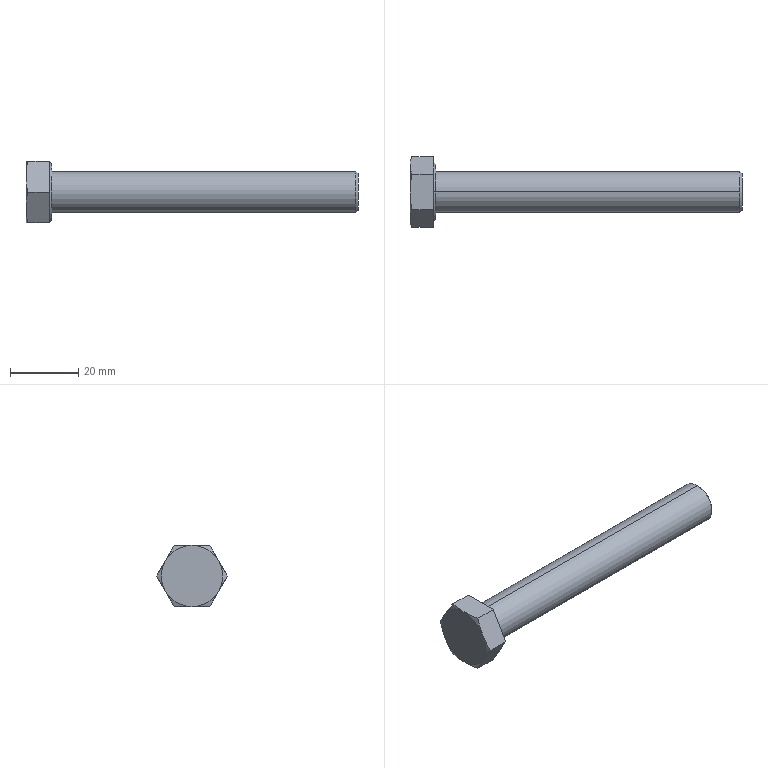Part | SolidWorks | features RevCut 3, Boss 1, Chamfer 1, Extrusion 1, Fillet 1, LPattern 1 | 1 solid | 22 faces | box 97.5 x 20.785 x 18 mm | volume 12242 mm3 | cone 10 | plane 10 | cylinder 2 | commonest cylinder face diameters 12 x2
STEP:
#1=CARTESIAN_POINT('',(97.5,0.,-5.4));
#2=VERTEX_POINT('',#1);
#3=CARTESIAN_POINT('',(97.5,0.,5.4));
#4=VERTEX_POINT('',#3);
#5=CARTESIAN_POINT('',(97.5,0.,0.));
#6=DIRECTION('',(1.,0.,0.));
#7=DIRECTION('',(0.,0.,-1.));
#8=AXIS2_PLACEMENT_3D('',#5,#6,#7);
#9=CIRCLE('',#8,5.4);
#10=EDGE_CURVE('',#2,#4,#9,.T.);
#11=ORIENTED_EDGE('',*,*,#10,.F.);
#12=CARTESIAN_POINT('',(96.9,0.,-6.));
#13=VERTEX_POINT('',#12);
#14=CARTESIAN_POINT('',(97.5,0.,-5.4));
#15=DIRECTION('',(-0.7071,0.,-0.7071));
#16=VECTOR('',#15,1000.);
#17=LINE('',#14,#16);
#18=EDGE_CURVE('',#2,#13,#17,.T.);
#19=ORIENTED_EDGE('',*,*,#18,.T.);
#20=CARTESIAN_POINT('',(96.9,0.,6.));
#21=VERTEX_POINT('',#20);
#22=CARTESIAN_POINT('',(96.9,0.,0.));
#23=DIRECTION('',(-1.,0.,0.));
#24=DIRECTION('',(0.,0.,-1.));
#25=AXIS2_PLACEMENT_3D('',#22,#23,#24);
#26=CIRCLE('',#25,6.);
#27=EDGE_CURVE('',#21,#13,#26,.T.);
#28=ORIENTED_EDGE('',*,*,#27,.F.);
#29=CARTESIAN_POINT('',(97.5,0.,5.4));
#30=DIRECTION('',(-0.7071,0.,0.7071));
#31=VECTOR('',#30,1000.);
#32=LINE('',#29,#31);
#33=EDGE_CURVE('',#4,#21,#32,.T.);
#34=ORIENTED_EDGE('',*,*,#33,.F.);
#35=EDGE_LOOP('',(#11,#19,#28,#34));
#36=FACE_OUTER_BOUND('',#35,.T.);
#37=CARTESIAN_POINT('',(97.5,0.,0.));
#38=DIRECTION('',(-1.,0.,0.));
#39=DIRECTION('',(0.,0.,1.));
#40=AXIS2_PLACEMENT_3D('',#37,#38,#39);
#41=CONICAL_SURFACE('',#40,5.4,0.7854);
#42=ADVANCED_FACE('',(#36),#41,.T.);
#43=ORIENTED_EDGE('',*,*,#27,.T.);
#44=CARTESIAN_POINT('',(7.5,0.,-6.));
#45=VERTEX_POINT('',#44);
#46=CARTESIAN_POINT('',(97.5,0.,-6.));
#47=DIRECTION('',(-1.,0.,0.));
#48=VECTOR('',#47,1000.);
#49=LINE('',#46,#48);
#50=EDGE_CURVE('',#13,#45,#49,.T.);
#51=ORIENTED_EDGE('',*,*,#50,.T.);
#52=CARTESIAN_POINT('',(7.5,0.,6.));
#53=VERTEX_POINT('',#52);
#54=CARTESIAN_POINT('',(7.5,0.,0.));
#55=DIRECTION('',(1.,0.,0.));
#56=DIRECTION('',(0.,0.,1.));
#57=AXIS2_PLACEMENT_3D('',#54,#55,#56);
#58=CIRCLE('',#57,6.);
#59=EDGE_CURVE('',#45,#53,#58,.T.);
#60=ORIENTED_EDGE('',*,*,#59,.T.);
#61=CARTESIAN_POINT('',(97.5,0.,6.));
#62=DIRECTION('',(-1.,0.,0.));
#63=VECTOR('',#62,1000.);
#64=LINE('',#61,#63);
#65=EDGE_CURVE('',#21,#53,#64,.T.);
#66=ORIENTED_EDGE('',*,*,#65,.F.);
#67=EDGE_LOOP('',(#43,#51,#60,#66));
#68=FACE_OUTER_BOUND('',#67,.T.);
#69=CARTESIAN_POINT('',(97.5,0.,0.));
#70=DIRECTION('',(-1.,0.,0.));
#71=DIRECTION('',(0.,0.,1.));
#72=AXIS2_PLACEMENT_3D('',#69,#70,#71);
#73=CYLINDRICAL_SURFACE('',#72,6.);
#74=ADVANCED_FACE('',(#68),#73,.T.);
#75=CARTESIAN_POINT('',(7.5,0.,8.235));
#76=VERTEX_POINT('',#75);
#77=CARTESIAN_POINT('',(7.5,0.,-8.235));
#78=VERTEX_POINT('',#77);
#79=CARTESIAN_POINT('',(7.5,0.,0.));
#80=DIRECTION('',(-1.,0.,0.));
#81=DIRECTION('',(0.,0.,1.));
#82=AXIS2_PLACEMENT_3D('',#79,#80,#81);
#83=CIRCLE('',#82,8.235);
#84=EDGE_CURVE('',#76,#78,#83,.T.);
#85=ORIENTED_EDGE('',*,*,#84,.T.);
#86=CARTESIAN_POINT('',(6.9,0.,-8.835));
#87=VERTEX_POINT('',#86);
#88=CARTESIAN_POINT('',(6.9,0.,-8.835));
#89=DIRECTION('',(-0.7071,0.,-0.7071));
#90=VECTOR('',#89,1000.);
#91=LINE('',#88,#90);
#92=EDGE_CURVE('',#78,#87,#91,.T.);
#93=ORIENTED_EDGE('',*,*,#92,.T.);
#94=CARTESIAN_POINT('',(6.9,0.,8.835));
#95=VERTEX_POINT('',#94);
#96=CARTESIAN_POINT('',(6.9,0.,0.));
#97=DIRECTION('',(-1.,0.,0.));
#98=DIRECTION('',(0.,0.,1.));
#99=AXIS2_PLACEMENT_3D('',#96,#97,#98);
#100=CIRCLE('',#99,8.835);
#101=EDGE_CURVE('',#95,#87,#100,.T.);
#102=ORIENTED_EDGE('',*,*,#101,.F.);
#103=CARTESIAN_POINT('',(6.9,0.,8.835));
#104=DIRECTION('',(-0.7071,0.,0.7071));
#105=VECTOR('',#104,1000.);
#106=LINE('',#103,#105);
#107=EDGE_CURVE('',#76,#95,#106,.T.);
#108=ORIENTED_EDGE('',*,*,#107,.F.);
#109=EDGE_LOOP('',(#85,#93,#102,#108));
#110=FACE_OUTER_BOUND('',#109,.T.);
#111=CARTESIAN_POINT('',(6.9,0.,0.));
#112=DIRECTION('',(-1.,0.,0.));
#113=DIRECTION('',(0.,0.,1.));
#114=AXIS2_PLACEMENT_3D('',#111,#112,#113);
#115=CONICAL_SURFACE('',#114,8.835,0.7854);
#116=ADVANCED_FACE('',(#110),#115,.T.);
#117=ORIENTED_EDGE('',*,*,#84,.F.);
#118=CARTESIAN_POINT('',(7.5,0.,0.));
#119=DIRECTION('',(-1.,0.,0.));
#120=DIRECTION('',(0.,0.,1.));
#121=AXIS2_PLACEMENT_3D('',#118,#119,#120);
#122=CIRCLE('',#121,8.235);
#123=EDGE_CURVE('',#78,#76,#122,.T.);
#124=ORIENTED_EDGE('',*,*,#123,.F.);
#125=EDGE_LOOP('',(#117,#124));
#126=FACE_OUTER_BOUND('',#125,.T.);
#127=CARTESIAN_POINT('',(7.5,0.,0.));
#128=DIRECTION('',(1.,0.,0.));
#129=DIRECTION('',(0.,0.,1.));
#130=AXIS2_PLACEMENT_3D('',#127,#128,#129);
#131=CIRCLE('',#130,6.);
#132=EDGE_CURVE('',#53,#45,#131,.T.);
#133=ORIENTED_EDGE('',*,*,#132,.F.);
#134=ORIENTED_EDGE('',*,*,#59,.F.);
#135=EDGE_LOOP('',(#133,#134));
#136=FACE_BOUND('',#135,.T.);
#137=CARTESIAN_POINT('',(7.5,-5.196,9.));
#138=DIRECTION('',(-1.,0.,0.));
#139=DIRECTION('',(0.,0.,1.));
#140=AXIS2_PLACEMENT_3D('',#137,#138,#139);
#141=PLANE('',#140);
#142=ADVANCED_FACE('',(#126,#136),#141,.F.);
#143=CARTESIAN_POINT('',(0.5068,-10.392,0.));
#144=VERTEX_POINT('',#143);
#145=CARTESIAN_POINT('',(0.,-7.794,4.5));
#146=VERTEX_POINT('',#145);
#147=CARTESIAN_POINT('',(0.5068,-10.392,0.));
#148=CARTESIAN_POINT('',(0.3492,-9.959,0.75));
#149=CARTESIAN_POINT('',(0.2212,-9.526,1.5));
#150=CARTESIAN_POINT('',(0.04634,-8.66,3.));
#151=CARTESIAN_POINT('',(0.,-8.227,3.75));
#152=CARTESIAN_POINT('',(0.,-7.794,4.5));
#153=B_SPLINE_CURVE_WITH_KNOTS('',3,(#147,#148,#149,#150,#151,#152),.UNSPECIFIED.,.F.,.F.,(4,2,4),(0.000000231,0.002598,0.005196),.UNSPECIFIED.);
#154=EDGE_CURVE('',#144,#146,#153,.T.);
#155=ORIENTED_EDGE('',*,*,#154,.F.);
#156=CARTESIAN_POINT('',(6.9,-10.392,0.));
#157=VERTEX_POINT('',#156);
#158=CARTESIAN_POINT('',(7.5,-10.392,0.));
#159=DIRECTION('',(-1.,0.,0.));
#160=VECTOR('',#159,1000.);
#161=LINE('',#158,#160);
#162=EDGE_CURVE('',#157,#144,#161,.T.);
#163=ORIENTED_EDGE('',*,*,#162,.F.);
#164=CARTESIAN_POINT('',(6.9,-5.196,9.));
#165=VERTEX_POINT('',#164);
#166=CARTESIAN_POINT('',(6.9,-5.196,9.));
#167=DIRECTION('',(0.,-0.5,-0.866));
#168=VECTOR('',#167,1000.);
#169=LINE('',#166,#168);
#170=EDGE_CURVE('',#165,#157,#169,.T.);
#171=ORIENTED_EDGE('',*,*,#170,.F.);
#172=CARTESIAN_POINT('',(0.5068,-5.196,9.));
#173=VERTEX_POINT('',#172);
#174=CARTESIAN_POINT('',(7.5,-5.196,9.));
#175=DIRECTION('',(-1.,0.,0.));
#176=VECTOR('',#175,1000.);
#177=LINE('',#174,#176);
#178=EDGE_CURVE('',#165,#173,#177,.T.);
#179=ORIENTED_EDGE('',*,*,#178,.T.);
#180=CARTESIAN_POINT('',(0.,-7.794,4.5));
#181=CARTESIAN_POINT('',(0.,-7.361,5.25));
#182=CARTESIAN_POINT('',(0.04634,-6.928,6.));
#183=CARTESIAN_POINT('',(0.2212,-6.062,7.5));
#184=CARTESIAN_POINT('',(0.3492,-5.629,8.25));
#185=CARTESIAN_POINT('',(0.5068,-5.196,9.));
#186=B_SPLINE_CURVE_WITH_KNOTS('',3,(#180,#181,#182,#183,#184,#185),.UNSPECIFIED.,.F.,.F.,(4,2,4),(0.005196,0.007794,0.01039),.UNSPECIFIED.);
#187=EDGE_CURVE('',#146,#173,#186,.T.);
#188=ORIENTED_EDGE('',*,*,#187,.F.);
#189=EDGE_LOOP('',(#155,#163,#171,#179,#188));
#190=FACE_OUTER_BOUND('',#189,.T.);
#191=CARTESIAN_POINT('',(7.5,-5.196,9.));
#192=DIRECTION('',(0.,0.866,-0.5));
#193=DIRECTION('',(0.,0.5,0.866));
#194=AXIS2_PLACEMENT_3D('',#191,#192,#193);
#195=PLANE('',#194);
#196=ADVANCED_FACE('',(#190),#195,.F.);
#197=CARTESIAN_POINT('',(0.5068,-5.196,-9.));
#198=VERTEX_POINT('',#197);
#199=CARTESIAN_POINT('',(0.,-7.794,-4.5));
#200=VERTEX_POINT('',#199);
#201=CARTESIAN_POINT('',(0.5068,-5.196,-9.));
#202=CARTESIAN_POINT('',(0.3492,-5.629,-8.25));
#203=CARTESIAN_POINT('',(0.2212,-6.062,-7.5));
#204=CARTESIAN_POINT('',(0.04634,-6.928,-6.));
#205=CARTESIAN_POINT('',(0.,-7.361,-5.25));
#206=CARTESIAN_POINT('',(0.,-7.794,-4.5));
#207=B_SPLINE_CURVE_WITH_KNOTS('',3,(#201,#202,#203,#204,#205,#206),.UNSPECIFIED.,.F.,.F.,(4,2,4),(0.000000231,0.002598,0.005196),.UNSPECIFIED.);
#208=EDGE_CURVE('',#198,#200,#207,.T.);
#209=ORIENTED_EDGE('',*,*,#208,.F.);
#210=CARTESIAN_POINT('',(6.9,-5.196,-9.));
#211=VERTEX_POINT('',#210);
#212=CARTESIAN_POINT('',(7.5,-5.196,-9.));
#213=DIRECTION('',(-1.,0.,0.));
#214=VECTOR('',#213,1000.);
#215=LINE('',#212,#214);
#216=EDGE_CURVE('',#211,#198,#215,.T.);
#217=ORIENTED_EDGE('',*,*,#216,.F.);
#218=CARTESIAN_POINT('',(6.9,-10.392,0.));
#219=DIRECTION('',(0.,0.5,-0.866));
#220=VECTOR('',#219,1000.);
#221=LINE('',#218,#220);
#222=EDGE_CURVE('',#157,#211,#221,.T.);
#223=ORIENTED_EDGE('',*,*,#222,.F.);
#224=ORIENTED_EDGE('',*,*,#162,.T.);
#225=CARTESIAN_POINT('',(0.,-7.794,-4.5));
#226=CARTESIAN_POINT('',(0.,-8.227,-3.75));
#227=CARTESIAN_POINT('',(0.04634,-8.66,-3.));
#228=CARTESIAN_POINT('',(0.2212,-9.526,-1.5));
#229=CARTESIAN_POINT('',(0.3492,-9.959,-0.75));
#230=CARTESIAN_POINT('',(0.5068,-10.392,0.));
#231=B_SPLINE_CURVE_WITH_KNOTS('',3,(#225,#226,#227,#228,#229,#230),.UNSPECIFIED.,.F.,.F.,(4,2,4),(0.005196,0.007794,0.01039),.UNSPECIFIED.);
#232=EDGE_CURVE('',#200,#144,#231,.T.);
#233=ORIENTED_EDGE('',*,*,#232,.F.);
#234=EDGE_LOOP('',(#209,#217,#223,#224,#233));
#235=FACE_OUTER_BOUND('',#234,.T.);
#236=CARTESIAN_POINT('',(7.5,-10.392,0.));
#237=DIRECTION('',(0.,0.866,0.5));
#238=DIRECTION('',(0.,-0.5,0.866));
#239=AXIS2_PLACEMENT_3D('',#236,#237,#238);
#240=PLANE('',#239);
#241=ADVANCED_FACE('',(#235),#240,.F.);
#242=CARTESIAN_POINT('',(0.5068,5.196,-9.));
#243=VERTEX_POINT('',#242);
#244=CARTESIAN_POINT('',(0.,0.,-9.));
#245=VERTEX_POINT('',#244);
#246=CARTESIAN_POINT('',(0.5068,5.196,-9.));
#247=CARTESIAN_POINT('',(0.3496,4.332,-9.));
#248=CARTESIAN_POINT('',(0.2215,3.467,-9.));
#249=CARTESIAN_POINT('',(0.04652,1.735,-9.));
#250=CARTESIAN_POINT('',(0.,0.8678,-9.));
#251=CARTESIAN_POINT('',(0.,0.,-9.));
#252=B_SPLINE_CURVE_WITH_KNOTS('',3,(#246,#247,#248,#249,#250,#251),.UNSPECIFIED.,.F.,.F.,(4,2,4),(0.01874,0.02136,0.02398),.UNSPECIFIED.);
#253=EDGE_CURVE('',#243,#245,#252,.T.);
#254=ORIENTED_EDGE('',*,*,#253,.F.);
#255=CARTESIAN_POINT('',(6.9,5.196,-9.));
#256=VERTEX_POINT('',#255);
#257=CARTESIAN_POINT('',(7.5,5.196,-9.));
#258=DIRECTION('',(-1.,0.,0.));
#259=VECTOR('',#258,1000.);
#260=LINE('',#257,#259);
#261=EDGE_CURVE('',#256,#243,#260,.T.);
#262=ORIENTED_EDGE('',*,*,#261,.F.);
#263=CARTESIAN_POINT('',(6.9,-5.196,-9.));
#264=DIRECTION('',(0.,1.,0.));
#265=VECTOR('',#264,1000.);
#266=LINE('',#263,#265);
#267=EDGE_CURVE('',#211,#256,#266,.T.);
#268=ORIENTED_EDGE('',*,*,#267,.F.);
#269=ORIENTED_EDGE('',*,*,#216,.T.);
#270=CARTESIAN_POINT('',(0.,0.,-9.));
#271=CARTESIAN_POINT('',(0.,-0.8653,-9.));
#272=CARTESIAN_POINT('',(0.04627,-1.732,-9.));
#273=CARTESIAN_POINT('',(0.2214,-3.466,-9.));
#274=CARTESIAN_POINT('',(0.3502,-4.336,-9.));
#275=CARTESIAN_POINT('',(0.5068,-5.196,-9.));
#276=B_SPLINE_CURVE_WITH_KNOTS('',3,(#270,#271,#272,#273,#274,#275),.UNSPECIFIED.,.F.,.F.,(4,2,4),(0.02398,0.02659,0.0292),.UNSPECIFIED.);
#277=EDGE_CURVE('',#245,#198,#276,.T.);
#278=ORIENTED_EDGE('',*,*,#277,.F.);
#279=EDGE_LOOP('',(#254,#262,#268,#269,#278));
#280=FACE_OUTER_BOUND('',#279,.T.);
#281=CARTESIAN_POINT('',(7.5,-5.196,-9.));
#282=DIRECTION('',(0.,0.,1.));
#283=DIRECTION('',(0.,-1.,0.));
#284=AXIS2_PLACEMENT_3D('',#281,#282,#283);
#285=PLANE('',#284);
#286=ADVANCED_FACE('',(#280),#285,.F.);
#287=CARTESIAN_POINT('',(0.5068,10.392,0.));
#288=VERTEX_POINT('',#287);
#289=CARTESIAN_POINT('',(0.,7.794,-4.5));
#290=VERTEX_POINT('',#289);
#291=CARTESIAN_POINT('',(0.5068,10.392,0.));
#292=CARTESIAN_POINT('',(0.3492,9.959,-0.75));
#293=CARTESIAN_POINT('',(0.2212,9.526,-1.5));
#294=CARTESIAN_POINT('',(0.04634,8.66,-3.));
#295=CARTESIAN_POINT('',(0.,8.227,-3.75));
#296=CARTESIAN_POINT('',(0.,7.794,-4.5));
#297=B_SPLINE_CURVE_WITH_KNOTS('',3,(#291,#292,#293,#294,#295,#296),.UNSPECIFIED.,.F.,.F.,(4,2,4),(0.000000231,0.002598,0.005196),.UNSPECIFIED.);
#298=EDGE_CURVE('',#288,#290,#297,.T.);
#299=ORIENTED_EDGE('',*,*,#298,.F.);
#300=CARTESIAN_POINT('',(6.9,10.392,0.));
#301=VERTEX_POINT('',#300);
#302=CARTESIAN_POINT('',(7.5,10.392,0.));
#303=DIRECTION('',(-1.,0.,0.));
#304=VECTOR('',#303,1000.);
#305=LINE('',#302,#304);
#306=EDGE_CURVE('',#301,#288,#305,.T.);
#307=ORIENTED_EDGE('',*,*,#306,.F.);
#308=CARTESIAN_POINT('',(6.9,5.196,-9.));
#309=DIRECTION('',(0.,0.5,0.866));
#310=VECTOR('',#309,1000.);
#311=LINE('',#308,#310);
#312=EDGE_CURVE('',#256,#301,#311,.T.);
#313=ORIENTED_EDGE('',*,*,#312,.F.);
#314=ORIENTED_EDGE('',*,*,#261,.T.);
#315=CARTESIAN_POINT('',(0.,7.794,-4.5));
#316=CARTESIAN_POINT('',(0.,7.361,-5.25));
#317=CARTESIAN_POINT('',(0.04634,6.928,-6.));
#318=CARTESIAN_POINT('',(0.2212,6.062,-7.5));
#319=CARTESIAN_POINT('',(0.3492,5.629,-8.25));
#320=CARTESIAN_POINT('',(0.5068,5.196,-9.));
#321=B_SPLINE_CURVE_WITH_KNOTS('',3,(#315,#316,#317,#318,#319,#320),.UNSPECIFIED.,.F.,.F.,(4,2,4),(0.005196,0.007794,0.01039),.UNSPECIFIED.);
#322=EDGE_CURVE('',#290,#243,#321,.T.);
#323=ORIENTED_EDGE('',*,*,#322,.F.);
#324=EDGE_LOOP('',(#299,#307,#313,#314,#323));
#325=FACE_OUTER_BOUND('',#324,.T.);
#326=CARTESIAN_POINT('',(7.5,5.196,-9.));
#327=DIRECTION('',(0.,-0.866,0.5));
#328=DIRECTION('',(0.,-0.5,-0.866));
#329=AXIS2_PLACEMENT_3D('',#326,#327,#328);
#330=PLANE('',#329);
#331=ADVANCED_FACE('',(#325),#330,.F.);
#332=CARTESIAN_POINT('',(0.5068,5.196,9.));
#333=VERTEX_POINT('',#332);
#334=CARTESIAN_POINT('',(0.,7.794,4.5));
#335=VERTEX_POINT('',#334);
#336=CARTESIAN_POINT('',(0.5068,5.196,9.));
#337=CARTESIAN_POINT('',(0.3492,5.629,8.25));
#338=CARTESIAN_POINT('',(0.2212,6.062,7.5));
#339=CARTESIAN_POINT('',(0.04634,6.928,6.));
#340=CARTESIAN_POINT('',(0.,7.361,5.25));
#341=CARTESIAN_POINT('',(0.,7.794,4.5));
#342=B_SPLINE_CURVE_WITH_KNOTS('',3,(#336,#337,#338,#339,#340,#341),.UNSPECIFIED.,.F.,.F.,(4,2,4),(0.000000231,0.002598,0.005196),.UNSPECIFIED.);
#343=EDGE_CURVE('',#333,#335,#342,.T.);
#344=ORIENTED_EDGE('',*,*,#343,.F.);
#345=CARTESIAN_POINT('',(6.9,5.196,9.));
#346=VERTEX_POINT('',#345);
#347=CARTESIAN_POINT('',(7.5,5.196,9.));
#348=DIRECTION('',(-1.,0.,0.));
#349=VECTOR('',#348,1000.);
#350=LINE('',#347,#349);
#351=EDGE_CURVE('',#346,#333,#350,.T.);
#352=ORIENTED_EDGE('',*,*,#351,.F.);
#353=CARTESIAN_POINT('',(6.9,10.392,0.));
#354=DIRECTION('',(0.,-0.5,0.866));
#355=VECTOR('',#354,1000.);
#356=LINE('',#353,#355);
#357=EDGE_CURVE('',#301,#346,#356,.T.);
#358=ORIENTED_EDGE('',*,*,#357,.F.);
#359=ORIENTED_EDGE('',*,*,#306,.T.);
#360=CARTESIAN_POINT('',(0.,7.794,4.5));
#361=CARTESIAN_POINT('',(0.,8.227,3.75));
#362=CARTESIAN_POINT('',(0.04634,8.66,3.));
#363=CARTESIAN_POINT('',(0.2212,9.526,1.5));
#364=CARTESIAN_POINT('',(0.3492,9.959,0.75));
#365=CARTESIAN_POINT('',(0.5068,10.392,0.));
#366=B_SPLINE_CURVE_WITH_KNOTS('',3,(#360,#361,#362,#363,#364,#365),.UNSPECIFIED.,.F.,.F.,(4,2,4),(0.005196,0.007794,0.01039),.UNSPECIFIED.);
#367=EDGE_CURVE('',#335,#288,#366,.T.);
#368=ORIENTED_EDGE('',*,*,#367,.F.);
#369=EDGE_LOOP('',(#344,#352,#358,#359,#368));
#370=FACE_OUTER_BOUND('',#369,.T.);
#371=CARTESIAN_POINT('',(7.5,10.392,0.));
#372=DIRECTION('',(0.,-0.866,-0.5));
#373=DIRECTION('',(0.,0.5,-0.866));
#374=AXIS2_PLACEMENT_3D('',#371,#372,#373);
#375=PLANE('',#374);
#376=ADVANCED_FACE('',(#370),#375,.F.);
#377=CARTESIAN_POINT('',(0.,0.,9.));
#378=VERTEX_POINT('',#377);
#379=CARTESIAN_POINT('',(0.5068,-5.196,9.));
#380=CARTESIAN_POINT('',(0.3502,-4.336,9.));
#381=CARTESIAN_POINT('',(0.2214,-3.466,9.));
#382=CARTESIAN_POINT('',(0.04627,-1.732,9.));
#383=CARTESIAN_POINT('',(0.,-0.8653,9.));
#384=CARTESIAN_POINT('',(0.,0.,9.));
#385=B_SPLINE_CURVE_WITH_KNOTS('',3,(#379,#380,#381,#382,#383,#384),.UNSPECIFIED.,.F.,.F.,(4,2,4),(0.008839,0.01146,0.01408),.UNSPECIFIED.);
#386=EDGE_CURVE('',#173,#378,#385,.T.);
#387=ORIENTED_EDGE('',*,*,#386,.F.);
#388=ORIENTED_EDGE('',*,*,#178,.F.);
#389=CARTESIAN_POINT('',(6.9,5.196,9.));
#390=DIRECTION('',(0.,-1.,0.));
#391=VECTOR('',#390,1000.);
#392=LINE('',#389,#391);
#393=EDGE_CURVE('',#346,#165,#392,.T.);
#394=ORIENTED_EDGE('',*,*,#393,.F.);
#395=ORIENTED_EDGE('',*,*,#351,.T.);
#396=CARTESIAN_POINT('',(0.,0.,9.));
#397=CARTESIAN_POINT('',(0.,0.8678,9.));
#398=CARTESIAN_POINT('',(0.04652,1.735,9.));
#399=CARTESIAN_POINT('',(0.2215,3.467,9.));
#400=CARTESIAN_POINT('',(0.3496,4.332,9.));
#401=CARTESIAN_POINT('',(0.5068,5.196,9.));
#402=B_SPLINE_CURVE_WITH_KNOTS('',3,(#396,#397,#398,#399,#400,#401),.UNSPECIFIED.,.F.,.F.,(4,2,4),(0.01408,0.0167,0.01933),.UNSPECIFIED.);
#403=EDGE_CURVE('',#378,#333,#402,.T.);
#404=ORIENTED_EDGE('',*,*,#403,.F.);
#405=EDGE_LOOP('',(#387,#388,#394,#395,#404));
#406=FACE_OUTER_BOUND('',#405,.T.);
#407=CARTESIAN_POINT('',(7.5,5.196,9.));
#408=DIRECTION('',(0.,0.,-1.));
#409=DIRECTION('',(-1.,0.,0.));
#410=AXIS2_PLACEMENT_3D('',#407,#408,#409);
#411=PLANE('',#410);
#412=ADVANCED_FACE('',(#406),#411,.F.);
#413=ORIENTED_EDGE('',*,*,#101,.T.);
#414=CARTESIAN_POINT('',(6.9,0.,0.));
#415=DIRECTION('',(-1.,0.,0.));
#416=DIRECTION('',(0.,0.,1.));
#417=AXIS2_PLACEMENT_3D('',#414,#415,#416);
#418=CIRCLE('',#417,8.835);
#419=EDGE_CURVE('',#87,#95,#418,.T.);
#420=ORIENTED_EDGE('',*,*,#419,.T.);
#421=EDGE_LOOP('',(#413,#420));
#422=FACE_BOUND('',#421,.T.);
#423=ORIENTED_EDGE('',*,*,#170,.T.);
#424=ORIENTED_EDGE('',*,*,#222,.T.);
#425=ORIENTED_EDGE('',*,*,#267,.T.);
#426=ORIENTED_EDGE('',*,*,#312,.T.);
#427=ORIENTED_EDGE('',*,*,#357,.T.);
#428=ORIENTED_EDGE('',*,*,#393,.T.);
#429=EDGE_LOOP('',(#423,#424,#425,#426,#427,#428));
#430=FACE_OUTER_BOUND('',#429,.T.);
#431=CARTESIAN_POINT('',(6.9,8.835,0.));
#432=DIRECTION('',(1.,0.,0.));
#433=DIRECTION('',(0.,0.,-1.));
#434=AXIS2_PLACEMENT_3D('',#431,#432,#433);
#435=PLANE('',#434);
#436=ADVANCED_FACE('',(#422,#430),#435,.T.);
#437=ORIENTED_EDGE('',*,*,#92,.F.);
#438=ORIENTED_EDGE('',*,*,#123,.T.);
#439=ORIENTED_EDGE('',*,*,#107,.T.);
#440=ORIENTED_EDGE('',*,*,#419,.F.);
#441=EDGE_LOOP('',(#437,#438,#439,#440));
#442=FACE_OUTER_BOUND('',#441,.T.);
#443=CARTESIAN_POINT('',(6.9,0.,0.));
#444=DIRECTION('',(-1.,0.,0.));
#445=DIRECTION('',(0.,0.,1.));
#446=AXIS2_PLACEMENT_3D('',#443,#444,#445);
#447=CONICAL_SURFACE('',#446,8.835,0.7854);
#448=ADVANCED_FACE('',(#442),#447,.T.);
#449=ORIENTED_EDGE('',*,*,#187,.T.);
#450=ORIENTED_EDGE('',*,*,#386,.T.);
#451=CARTESIAN_POINT('',(0.,0.,0.));
#452=DIRECTION('',(-1.,0.,0.));
#453=DIRECTION('',(0.,0.,1.));
#454=AXIS2_PLACEMENT_3D('',#451,#452,#453);
#455=CIRCLE('',#454,9.);
#456=EDGE_CURVE('',#146,#378,#455,.T.);
#457=ORIENTED_EDGE('',*,*,#456,.F.);
#458=EDGE_LOOP('',(#449,#450,#457));
#459=FACE_OUTER_BOUND('',#458,.T.);
#460=CARTESIAN_POINT('',(0.,0.,0.));
#461=DIRECTION('',(1.,0.,0.));
#462=DIRECTION('',(0.,0.,-1.));
#463=AXIS2_PLACEMENT_3D('',#460,#461,#462);
#464=CONICAL_SURFACE('',#463,9.,1.222);
#465=ADVANCED_FACE('',(#459),#464,.T.);
#466=ORIENTED_EDGE('',*,*,#232,.T.);
#467=ORIENTED_EDGE('',*,*,#154,.T.);
#468=CARTESIAN_POINT('',(0.,0.,0.));
#469=DIRECTION('',(-1.,0.,0.));
#470=DIRECTION('',(0.,0.,1.));
#471=AXIS2_PLACEMENT_3D('',#468,#469,#470);
#472=CIRCLE('',#471,9.);
#473=EDGE_CURVE('',#200,#146,#472,.T.);
#474=ORIENTED_EDGE('',*,*,#473,.F.);
#475=EDGE_LOOP('',(#466,#467,#474));
#476=FACE_OUTER_BOUND('',#475,.T.);
#477=CARTESIAN_POINT('',(0.,0.,0.));
#478=DIRECTION('',(1.,0.,0.));
#479=DIRECTION('',(0.,0.,-1.));
#480=AXIS2_PLACEMENT_3D('',#477,#478,#479);
#481=CONICAL_SURFACE('',#480,9.,1.222);
#482=ADVANCED_FACE('',(#476),#481,.T.);
#483=ORIENTED_EDGE('',*,*,#277,.T.);
#484=ORIENTED_EDGE('',*,*,#208,.T.);
#485=CARTESIAN_POINT('',(0.,0.,0.));
#486=DIRECTION('',(-1.,0.,0.));
#487=DIRECTION('',(0.,0.,1.));
#488=AXIS2_PLACEMENT_3D('',#485,#486,#487);
#489=CIRCLE('',#488,9.);
#490=EDGE_CURVE('',#245,#200,#489,.T.);
#491=ORIENTED_EDGE('',*,*,#490,.F.);
#492=EDGE_LOOP('',(#483,#484,#491));
#493=FACE_OUTER_BOUND('',#492,.T.);
#494=CARTESIAN_POINT('',(0.,0.,0.));
#495=DIRECTION('',(1.,0.,0.));
#496=DIRECTION('',(0.,0.,-1.));
#497=AXIS2_PLACEMENT_3D('',#494,#495,#496);
#498=CONICAL_SURFACE('',#497,9.,1.222);
#499=ADVANCED_FACE('',(#493),#498,.T.);
#500=ORIENTED_EDGE('',*,*,#253,.T.);
#501=CARTESIAN_POINT('',(0.,0.,0.));
#502=DIRECTION('',(-1.,0.,0.));
#503=DIRECTION('',(0.,0.,1.));
#504=AXIS2_PLACEMENT_3D('',#501,#502,#503);
#505=CIRCLE('',#504,9.);
#506=EDGE_CURVE('',#290,#245,#505,.T.);
#507=ORIENTED_EDGE('',*,*,#506,.F.);
#508=ORIENTED_EDGE('',*,*,#322,.T.);
#509=EDGE_LOOP('',(#500,#507,#508));
#510=FACE_OUTER_BOUND('',#509,.T.);
#511=CARTESIAN_POINT('',(0.,0.,0.));
#512=DIRECTION('',(1.,0.,0.));
#513=DIRECTION('',(0.,0.,-1.));
#514=AXIS2_PLACEMENT_3D('',#511,#512,#513);
#515=CONICAL_SURFACE('',#514,9.,1.222);
#516=ADVANCED_FACE('',(#510),#515,.T.);
#517=ORIENTED_EDGE('',*,*,#298,.T.);
#518=CARTESIAN_POINT('',(0.,0.,0.));
#519=DIRECTION('',(-1.,0.,0.));
#520=DIRECTION('',(0.,0.,1.));
#521=AXIS2_PLACEMENT_3D('',#518,#519,#520);
#522=CIRCLE('',#521,9.);
#523=EDGE_CURVE('',#335,#290,#522,.T.);
#524=ORIENTED_EDGE('',*,*,#523,.F.);
#525=ORIENTED_EDGE('',*,*,#367,.T.);
#526=EDGE_LOOP('',(#517,#524,#525));
#527=FACE_OUTER_BOUND('',#526,.T.);
#528=CARTESIAN_POINT('',(0.,0.,0.));
#529=DIRECTION('',(1.,0.,0.));
#530=DIRECTION('',(0.,0.,-1.));
#531=AXIS2_PLACEMENT_3D('',#528,#529,#530);
#532=CONICAL_SURFACE('',#531,9.,1.222);
#533=ADVANCED_FACE('',(#527),#532,.T.);
#534=ORIENTED_EDGE('',*,*,#343,.T.);
#535=CARTESIAN_POINT('',(0.,0.,0.));
#536=DIRECTION('',(-1.,0.,0.));
#537=DIRECTION('',(0.,0.,1.));
#538=AXIS2_PLACEMENT_3D('',#535,#536,#537);
#539=CIRCLE('',#538,9.);
#540=EDGE_CURVE('',#378,#335,#539,.T.);
#541=ORIENTED_EDGE('',*,*,#540,.F.);
#542=ORIENTED_EDGE('',*,*,#403,.T.);
#543=EDGE_LOOP('',(#534,#541,#542));
#544=FACE_OUTER_BOUND('',#543,.T.);
#545=CARTESIAN_POINT('',(0.,0.,0.));
#546=DIRECTION('',(1.,0.,0.));
#547=DIRECTION('',(0.,0.,-1.));
#548=AXIS2_PLACEMENT_3D('',#545,#546,#547);
#549=CONICAL_SURFACE('',#548,9.,1.222);
#550=ADVANCED_FACE('',(#544),#549,.T.);
#551=ORIENTED_EDGE('',*,*,#456,.T.);
#552=ORIENTED_EDGE('',*,*,#540,.T.);
#553=ORIENTED_EDGE('',*,*,#523,.T.);
#554=ORIENTED_EDGE('',*,*,#506,.T.);
#555=ORIENTED_EDGE('',*,*,#490,.T.);
#556=ORIENTED_EDGE('',*,*,#473,.T.);
#557=EDGE_LOOP('',(#551,#552,#553,#554,#555,#556));
#558=FACE_OUTER_BOUND('',#557,.T.);
#559=CARTESIAN_POINT('',(0.,-5.196,9.));
#560=DIRECTION('',(-1.,0.,0.));
#561=DIRECTION('',(0.,0.,1.));
#562=AXIS2_PLACEMENT_3D('',#559,#560,#561);
#563=PLANE('',#562);
#564=ADVANCED_FACE('',(#558),#563,.T.);
#565=ORIENTED_EDGE('',*,*,#50,.F.);
#566=CARTESIAN_POINT('',(96.9,0.,0.));
#567=DIRECTION('',(-1.,0.,0.));
#568=DIRECTION('',(0.,0.,-1.));
#569=AXIS2_PLACEMENT_3D('',#566,#567,#568);
#570=CIRCLE('',#569,6.);
#571=EDGE_CURVE('',#13,#21,#570,.T.);
#572=ORIENTED_EDGE('',*,*,#571,.T.);
#573=ORIENTED_EDGE('',*,*,#65,.T.);
#574=ORIENTED_EDGE('',*,*,#132,.T.);
#575=EDGE_LOOP('',(#565,#572,#573,#574));
#576=FACE_OUTER_BOUND('',#575,.T.);
#577=CARTESIAN_POINT('',(97.5,0.,0.));
#578=DIRECTION('',(-1.,0.,0.));
#579=DIRECTION('',(0.,0.,1.));
#580=AXIS2_PLACEMENT_3D('',#577,#578,#579);
#581=CYLINDRICAL_SURFACE('',#580,6.);
#582=ADVANCED_FACE('',(#576),#581,.T.);
#583=CARTESIAN_POINT('',(97.5,0.,0.));
#584=DIRECTION('',(1.,0.,0.));
#585=DIRECTION('',(0.,0.,-1.));
#586=AXIS2_PLACEMENT_3D('',#583,#584,#585);
#587=CIRCLE('',#586,5.4);
#588=EDGE_CURVE('',#4,#2,#587,.T.);
#589=ORIENTED_EDGE('',*,*,#588,.T.);
#590=ORIENTED_EDGE('',*,*,#10,.T.);
#591=EDGE_LOOP('',(#589,#590));
#592=FACE_OUTER_BOUND('',#591,.T.);
#593=CARTESIAN_POINT('',(97.5,0.,0.));
#594=DIRECTION('',(1.,0.,0.));
#595=DIRECTION('',(0.,0.,-1.));
#596=AXIS2_PLACEMENT_3D('',#593,#594,#595);
#597=PLANE('',#596);
#598=ADVANCED_FACE('',(#592),#597,.T.);
#599=ORIENTED_EDGE('',*,*,#18,.F.);
#600=ORIENTED_EDGE('',*,*,#588,.F.);
#601=ORIENTED_EDGE('',*,*,#33,.T.);
#602=ORIENTED_EDGE('',*,*,#571,.F.);
#603=EDGE_LOOP('',(#599,#600,#601,#602));
#604=FACE_OUTER_BOUND('',#603,.T.);
#605=CARTESIAN_POINT('',(97.5,0.,0.));
#606=DIRECTION('',(-1.,0.,0.));
#607=DIRECTION('',(0.,0.,1.));
#608=AXIS2_PLACEMENT_3D('',#605,#606,#607);
#609=CONICAL_SURFACE('',#608,5.4,0.7854);
#610=ADVANCED_FACE('',(#604),#609,.T.);
#611=CLOSED_SHELL('',(#42,#74,#116,#142,#196,#241,#286,#331,#376,#412,#436,#448,#465,#482,#499,#516,#533,#550,#564,#582,#598,#610));
#612=MANIFOLD_SOLID_BREP('',#611);
#613=CARTESIAN_POINT('',(0.,0.,0.));
#614=DIRECTION('',(0.,0.,1.));
#615=DIRECTION('',(1.,0.,0.));
#616=AXIS2_PLACEMENT_3D('',#613,#614,#615);
#617=(LENGTH_UNIT()NAMED_UNIT(*)SI_UNIT(.MILLI.,.METRE.));
#618=UNCERTAINTY_MEASURE_WITH_UNIT(LENGTH_MEASURE(0.00001),#617,'','');
#619=(NAMED_UNIT(*)PLANE_ANGLE_UNIT()SI_UNIT($,.RADIAN.));
#620=(NAMED_UNIT(*)SI_UNIT($,.STERADIAN.)SOLID_ANGLE_UNIT());
#621=(GEOMETRIC_REPRESENTATION_CONTEXT(3)GLOBAL_UNCERTAINTY_ASSIGNED_CONTEXT((#618))GLOBAL_UNIT_ASSIGNED_CONTEXT((#617,#619,#620))REPRESENTATION_CONTEXT('',''));
#622=ADVANCED_BREP_SHAPE_REPRESENTATION('',(#612,#616),#621);